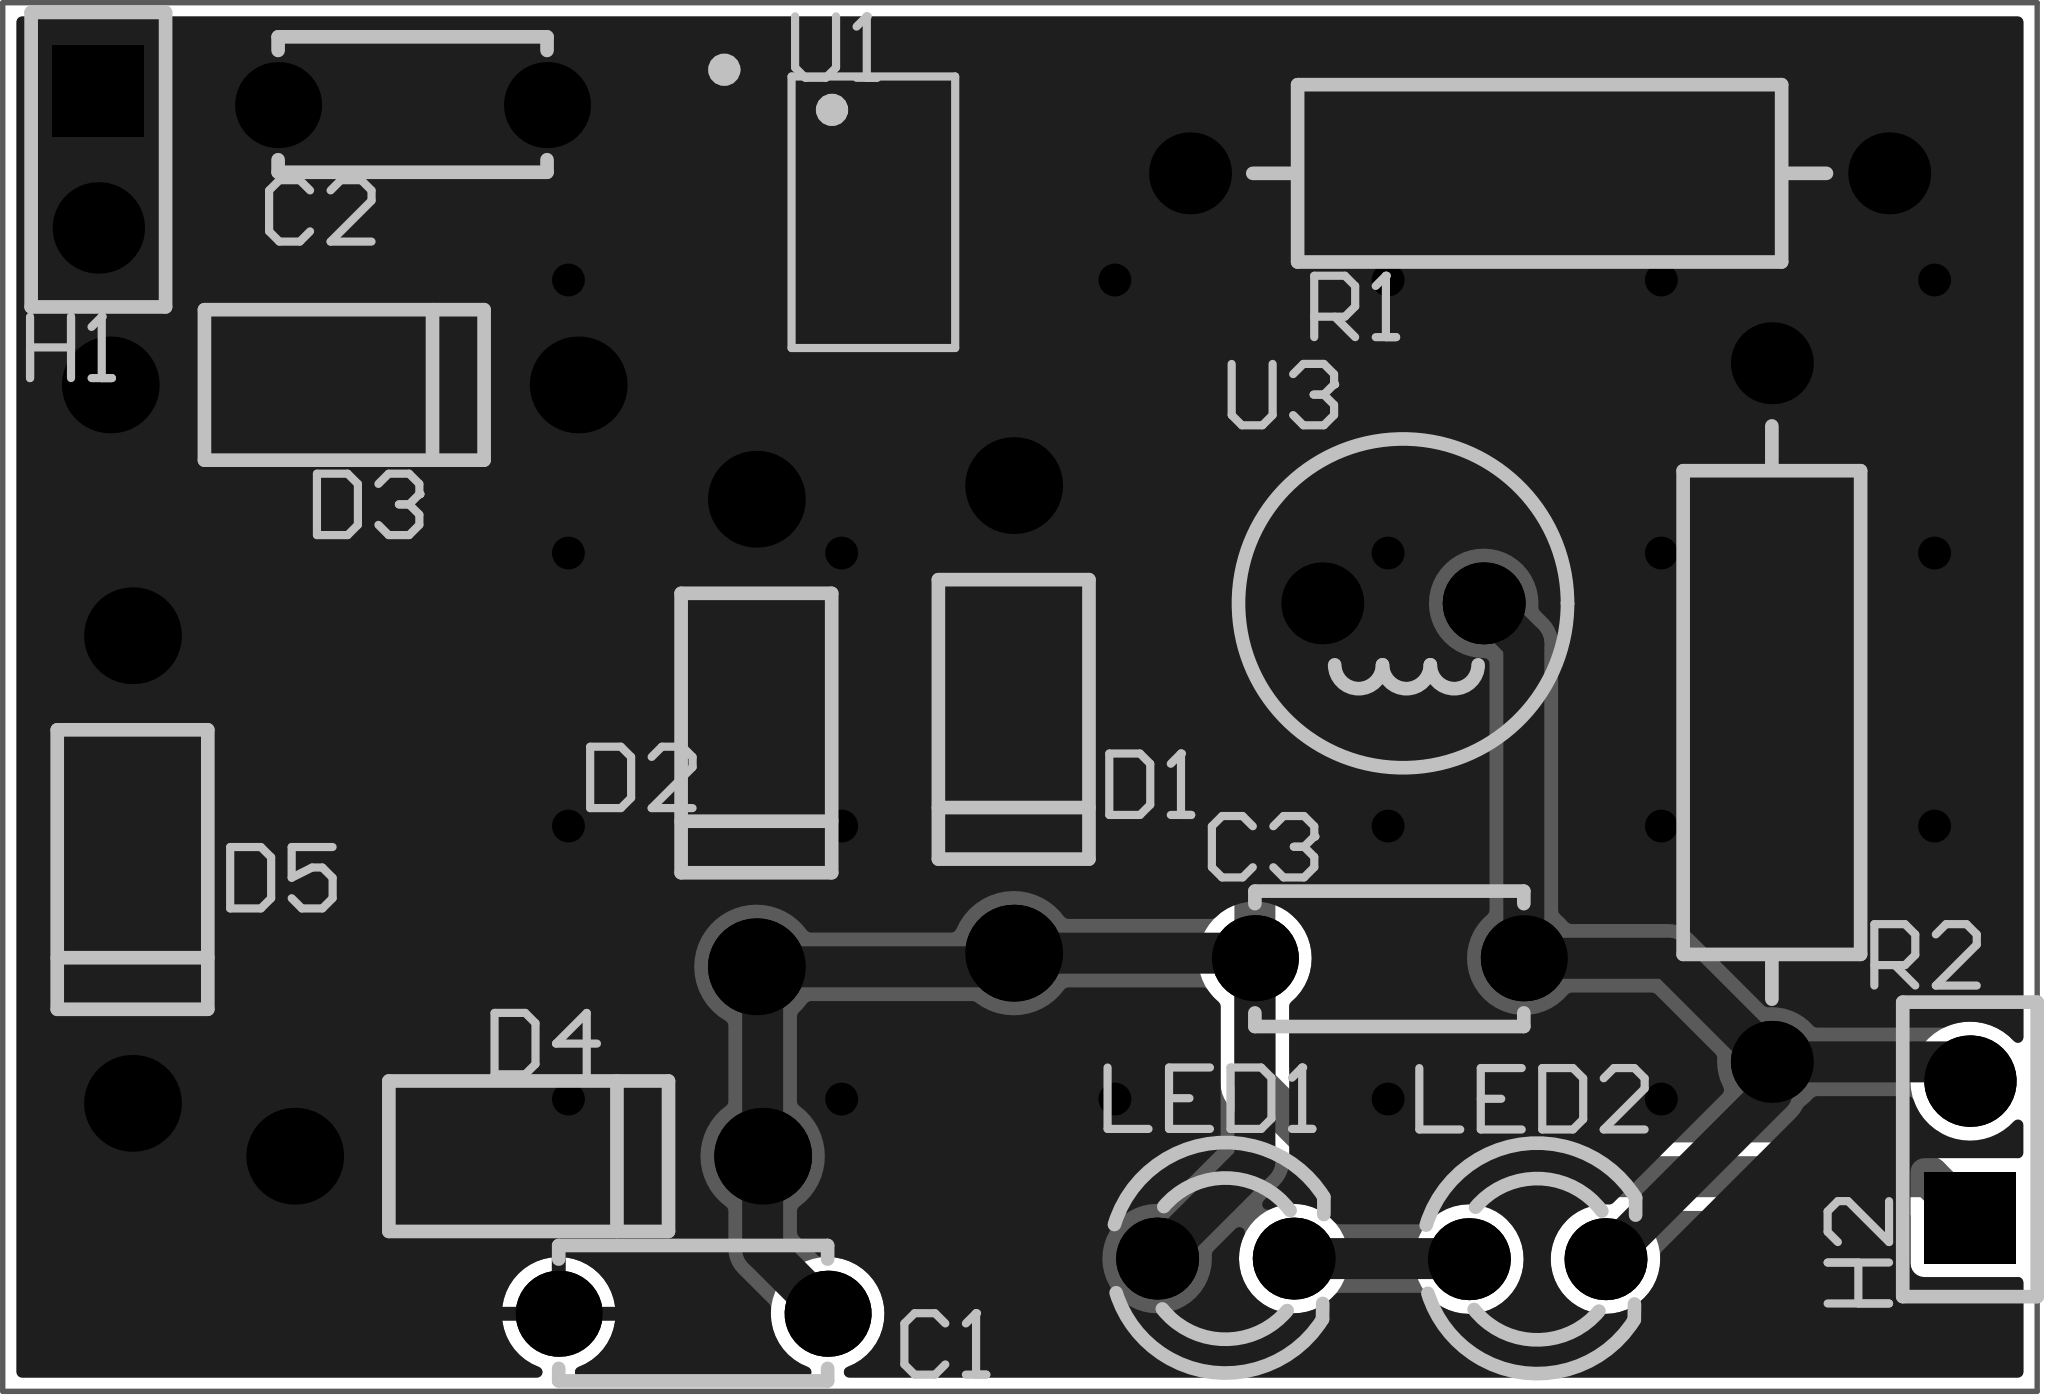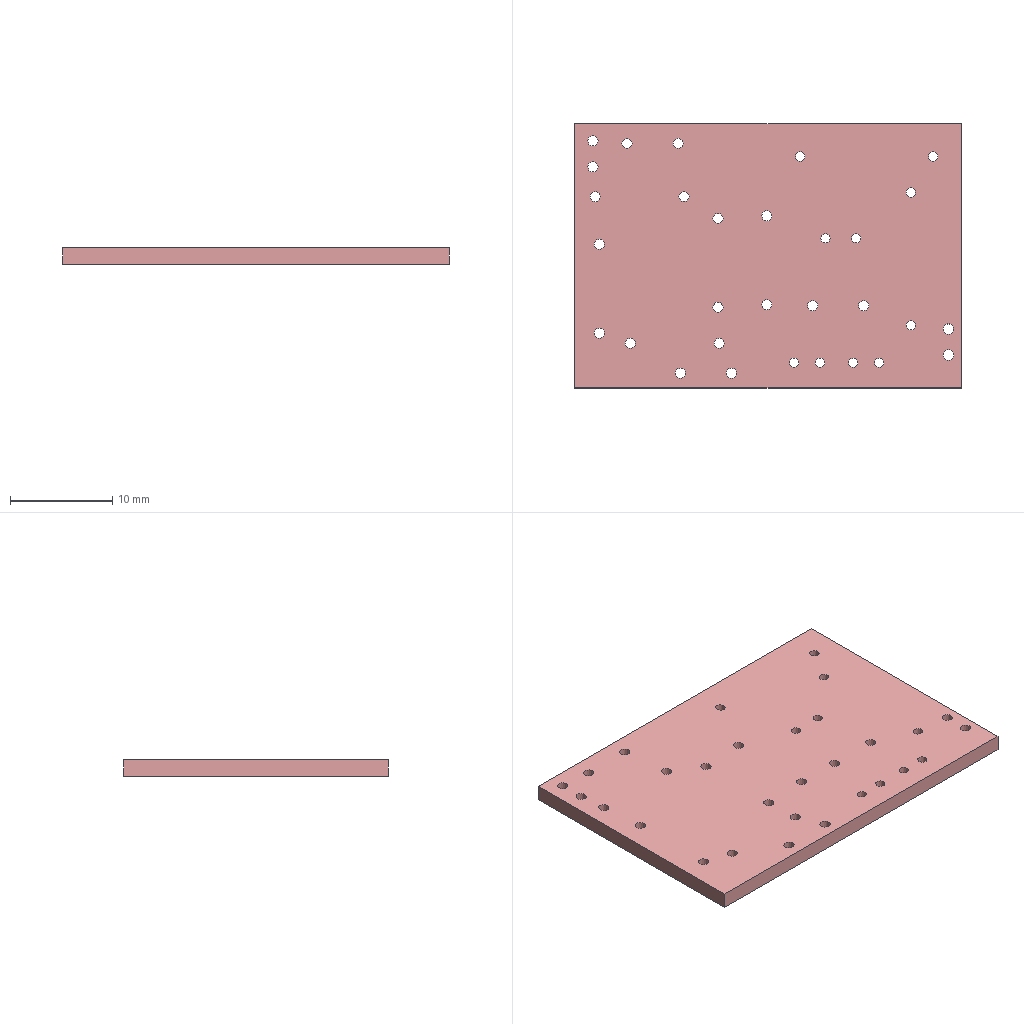Circuit board layout | Altium Designer | box 37.8 x 25.8 x 1.6 mm
Layer stack:
# Altium Designer layer stack of  (unit mm; dielectric type: 0 none, 1 core, 2 prepreg, 3 surface material)
index,name,kind,layer,copper_thickness_mm,dielectric_type,dielectric_thickness_mm,dielectric_material,dielectric_constant
0,Top Paste Mask Layer,other,,,,,,
1,Top Silkscreen Layer,other,,,,,,
2,Top Solder Mask Layer,dielectric,,,3,0.01,,3.3
3,Top Layer,copper,Top Layer,0.035,,,,
4,Dielectric1,dielectric,,,3,1.51,FR4,4.5
5,Bottom Layer,copper,Bottom Layer,0.035,,,,
6,Bottom Solder Mask Layer,dielectric,,,3,0.01,,3.3
7,Bottom Silkscreen Layer,other,,,,,,
8,Bottom Paste Mask Layer,other,,,,,,
# drill layer pairs: low layer,high layer
drill_pair,Top Layer,Bottom Layer
Part placement:
Designator,Comment,Layer,Footprint,Center-X(mm),Center-Y(mm),Rotation
C2,100nF,TopLayer,CAP-TH_L5.0-W2.5-P5.00-D1.0,88.519,103.759,180
C3,100nF,TopLayer,CAP-TH_L5.0-W2.5-P5.00-D1.0,106.68,87.884,0
D1,,TopLayer,DO_1N4007,99.695,92.329,90
D2,,TopLayer,DO_1N4007,94.912,92.075,90
D3,,TopLayer,DO_1N4007,87.249,98.552,180
D4,,TopLayer,DO_1N4007,90.678,84.201,180
D5,,TopLayer,DO_1N4007,83.312,89.535,90
H1,,TopLayer,HDR-TH_2P-P2.54-V-F,82.677,102.743,270
H2,,TopLayer,HDR-TH_2P-P2.54-V-F,117.475,84.328,90
LED1,,TopLayer,LED_TH-3mm,103.632,82.296,0
LED2,,TopLayer,LED_TH-3mm,109.428,82.285,0
R1,10kO,TopLayer,Res_1/2W,109.474,102.489,0
R2,10kO,TopLayer,Res_1/2W,113.792,92.456,90
U1,PT4501C,TopLayer,SOP-8_L4.9-W3.9-P1.27-LS6.0-BL-EP,97.087,101.765,270
U3,L6_8MM,TopLayer,IND-TH_BD6.00-P3.00-D0.6,106.934,94.488,0
C1,100nF,TopLayer,CAP-TH_L5.0-W2.5-P5.00-D1.0,93.736,81.27,180
Pad and via stacks:
# Altium Designer via and pad stacks of  (unit mm). Each distinct definition once, with the count of objects using it.
# via: kind,start_layer,end_layer,hole_mm,diameter_mm,mode(0 simple;1 top-mid-bottom;2 full stack),diameter_per_layer,count,example_net
# pad: kind,layer,hole_mm,hole_type(0 round;1 square;2 slot),plating,top_size,top_shape(1 round;2 rect;3 octagon;9 rounded rect),mid_size,bottom_size,mode,footprint,size_per_layer,count,example
pad,Multi-Layer,1,0,plated,1.6x1.6,1,1.6x1.6,1.6x1.6,0,CAP-TH_L5.0-W2.5-P5.00-D1.0,,6,C2.1
pad,Multi-Layer,1,0,plated,1.8x1.8,1,1.8x1.8,1.8x1.8,0,DO_1N4007,,10,D1.1
pad,Multi-Layer,1,0,plated,1.7x1.7,2,1.7x1.7,1.7x1.7,0,HDR-TH_2P-P2.54-V-F,,2,H1.1
pad,Multi-Layer,1,0,plated,1.7x1.7,1,1.7x1.7,1.7x1.7,0,HDR-TH_2P-P2.54-V-F,,2,H1.2
pad,Multi-Layer,0.9144,0,plated,1.524x1.524,1,1.524x1.524,1.524x1.524,0,LED_TH-3mm,,4,LED1.1
pad,Multi-Layer,0.9144,0,plated,1.524x1.524,1,1.524x1.524,1.524x1.524,0,Res_1/2W,,4,R1.2
pad,Multi-Layer,0.9144,0,plated,1.524x1.524,1,1.524x1.524,1.524x1.524,0,IND-TH_BD6.00-P3.00-D0.6,,2,U3.1
pad,Top Layer,0,0,plated,0.6x1.8,1,0.6x1.8,0.6x1.8,0,SOP-8_L4.9-W3.9-P1.27-LS6.0-BL-EP,,8,U1.1
via,Top Layer,Bottom Layer,0.3048,0.61,0,,20,GND
Copper pours:
name,layer,net,type(0 solid;1 hatched;2 none)
Bottom Layer-GND,Bottom Layer,GND,0
Top Layer-GND,Top Layer,GND,0